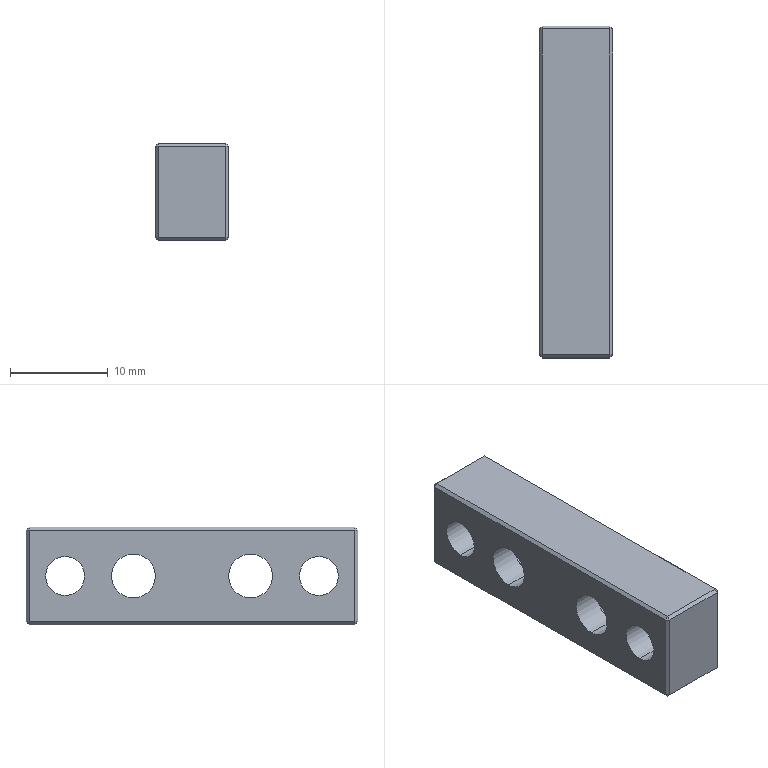Part | STEP file | A038 | 1 solid | 40 faces | box 7.5 x 34 x 10 mm | volume 1805 mm3 | plane 28 | cylinder 12 | commonest cylinder face diameters 4 x4 4.5 x4 8 x4